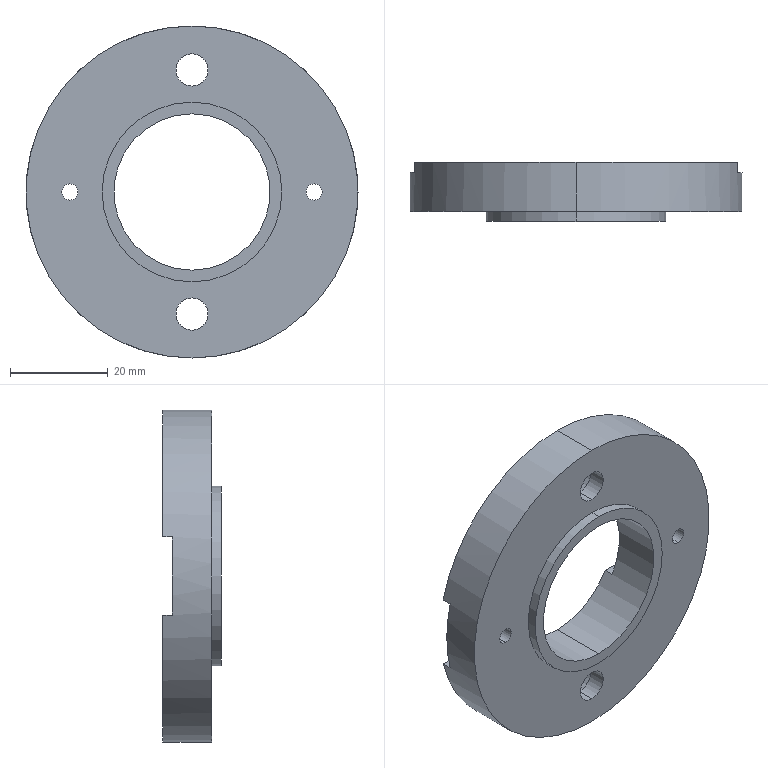Part | SolidWorks | features ICE 6, HoleWzd 2, Revolution 1 | 1 solid | 30 faces | box 68 x 12 x 68 mm | volume 26017 mm3 | cylinder 18 | plane 12 | commonest cylinder face diameters 3.3 x4 6.6 x4 11 x4 32 x2 36.8 x2 68 x2
STEP:
#1=CARTESIAN_POINT('',(-25.,36.,1.65));
#2=VERTEX_POINT('',#1);
#3=CARTESIAN_POINT('',(-25.,36.,-1.65));
#4=VERTEX_POINT('',#3);
#5=CARTESIAN_POINT('',(-25.,36.,0.));
#6=DIRECTION('',(0.,-1.,0.));
#7=DIRECTION('',(0.,0.,-1.));
#8=AXIS2_PLACEMENT_3D('',#5,#6,#7);
#9=CIRCLE('',#8,1.65);
#10=EDGE_CURVE('',#2,#4,#9,.T.);
#11=ORIENTED_EDGE('',*,*,#10,.T.);
#12=CARTESIAN_POINT('',(-25.,44.,-1.65));
#13=VERTEX_POINT('',#12);
#14=CARTESIAN_POINT('',(-25.,46.,-1.65));
#15=DIRECTION('',(0.,1.,0.));
#16=VECTOR('',#15,1000.);
#17=LINE('',#14,#16);
#18=EDGE_CURVE('',#4,#13,#17,.T.);
#19=ORIENTED_EDGE('',*,*,#18,.T.);
#20=CARTESIAN_POINT('',(-25.,44.,1.65));
#21=VERTEX_POINT('',#20);
#22=CARTESIAN_POINT('',(-25.,44.,0.));
#23=DIRECTION('',(0.,1.,0.));
#24=DIRECTION('',(0.,0.,1.));
#25=AXIS2_PLACEMENT_3D('',#22,#23,#24);
#26=CIRCLE('',#25,1.65);
#27=EDGE_CURVE('',#13,#21,#26,.T.);
#28=ORIENTED_EDGE('',*,*,#27,.T.);
#29=CARTESIAN_POINT('',(-25.,46.,1.65));
#30=DIRECTION('',(0.,1.,0.));
#31=VECTOR('',#30,1000.);
#32=LINE('',#29,#31);
#33=EDGE_CURVE('',#2,#21,#32,.T.);
#34=ORIENTED_EDGE('',*,*,#33,.F.);
#35=EDGE_LOOP('',(#11,#19,#28,#34));
#36=FACE_OUTER_BOUND('',#35,.T.);
#37=CARTESIAN_POINT('',(-25.,46.,0.));
#38=DIRECTION('',(0.,1.,0.));
#39=DIRECTION('',(0.,0.,1.));
#40=AXIS2_PLACEMENT_3D('',#37,#38,#39);
#41=CYLINDRICAL_SURFACE('',#40,1.65);
#42=ADVANCED_FACE('',(#36),#41,.F.);
#43=CARTESIAN_POINT('',(25.,36.,1.65));
#44=VERTEX_POINT('',#43);
#45=CARTESIAN_POINT('',(25.,36.,-1.65));
#46=VERTEX_POINT('',#45);
#47=CARTESIAN_POINT('',(25.,36.,0.));
#48=DIRECTION('',(0.,-1.,0.));
#49=DIRECTION('',(0.,0.,-1.));
#50=AXIS2_PLACEMENT_3D('',#47,#48,#49);
#51=CIRCLE('',#50,1.65);
#52=EDGE_CURVE('',#44,#46,#51,.T.);
#53=ORIENTED_EDGE('',*,*,#52,.T.);
#54=CARTESIAN_POINT('',(25.,44.,-1.65));
#55=VERTEX_POINT('',#54);
#56=CARTESIAN_POINT('',(25.,46.,-1.65));
#57=DIRECTION('',(0.,1.,0.));
#58=VECTOR('',#57,1000.);
#59=LINE('',#56,#58);
#60=EDGE_CURVE('',#46,#55,#59,.T.);
#61=ORIENTED_EDGE('',*,*,#60,.T.);
#62=CARTESIAN_POINT('',(25.,44.,1.65));
#63=VERTEX_POINT('',#62);
#64=CARTESIAN_POINT('',(25.,44.,0.));
#65=DIRECTION('',(0.,1.,0.));
#66=DIRECTION('',(0.,0.,1.));
#67=AXIS2_PLACEMENT_3D('',#64,#65,#66);
#68=CIRCLE('',#67,1.65);
#69=EDGE_CURVE('',#55,#63,#68,.T.);
#70=ORIENTED_EDGE('',*,*,#69,.T.);
#71=CARTESIAN_POINT('',(25.,46.,1.65));
#72=DIRECTION('',(0.,1.,0.));
#73=VECTOR('',#72,1000.);
#74=LINE('',#71,#73);
#75=EDGE_CURVE('',#44,#63,#74,.T.);
#76=ORIENTED_EDGE('',*,*,#75,.F.);
#77=EDGE_LOOP('',(#53,#61,#70,#76));
#78=FACE_OUTER_BOUND('',#77,.T.);
#79=CARTESIAN_POINT('',(25.,46.,0.));
#80=DIRECTION('',(0.,1.,0.));
#81=DIRECTION('',(0.,0.,1.));
#82=AXIS2_PLACEMENT_3D('',#79,#80,#81);
#83=CYLINDRICAL_SURFACE('',#82,1.65);
#84=ADVANCED_FACE('',(#78),#83,.F.);
#85=CARTESIAN_POINT('',(0.,39.6,-30.5));
#86=VERTEX_POINT('',#85);
#87=CARTESIAN_POINT('',(0.,39.6,-19.5));
#88=VERTEX_POINT('',#87);
#89=CARTESIAN_POINT('',(0.,39.6,-25.));
#90=DIRECTION('',(0.,1.,0.));
#91=DIRECTION('',(0.,0.,1.));
#92=AXIS2_PLACEMENT_3D('',#89,#90,#91);
#93=CIRCLE('',#92,5.5);
#94=EDGE_CURVE('',#86,#88,#93,.T.);
#95=ORIENTED_EDGE('',*,*,#94,.F.);
#96=CARTESIAN_POINT('',(0.,46.,-30.5));
#97=VERTEX_POINT('',#96);
#98=CARTESIAN_POINT('',(0.,46.,-30.5));
#99=DIRECTION('',(0.,1.,0.));
#100=VECTOR('',#99,1000.);
#101=LINE('',#98,#100);
#102=EDGE_CURVE('',#86,#97,#101,.T.);
#103=ORIENTED_EDGE('',*,*,#102,.T.);
#104=CARTESIAN_POINT('',(0.,46.,-19.5));
#105=VERTEX_POINT('',#104);
#106=CARTESIAN_POINT('',(0.,46.,-25.));
#107=DIRECTION('',(0.,1.,0.));
#108=DIRECTION('',(0.,0.,1.));
#109=AXIS2_PLACEMENT_3D('',#106,#107,#108);
#110=CIRCLE('',#109,5.5);
#111=EDGE_CURVE('',#97,#105,#110,.T.);
#112=ORIENTED_EDGE('',*,*,#111,.T.);
#113=CARTESIAN_POINT('',(0.,46.,-19.5));
#114=DIRECTION('',(0.,1.,0.));
#115=VECTOR('',#114,1000.);
#116=LINE('',#113,#115);
#117=EDGE_CURVE('',#88,#105,#116,.T.);
#118=ORIENTED_EDGE('',*,*,#117,.F.);
#119=EDGE_LOOP('',(#95,#103,#112,#118));
#120=FACE_OUTER_BOUND('',#119,.T.);
#121=CARTESIAN_POINT('',(0.,46.,-25.));
#122=DIRECTION('',(0.,1.,0.));
#123=DIRECTION('',(0.,0.,1.));
#124=AXIS2_PLACEMENT_3D('',#121,#122,#123);
#125=CYLINDRICAL_SURFACE('',#124,5.5);
#126=ADVANCED_FACE('',(#120),#125,.F.);
#127=CARTESIAN_POINT('',(0.,36.,-21.7));
#128=VERTEX_POINT('',#127);
#129=CARTESIAN_POINT('',(0.,36.,-28.3));
#130=VERTEX_POINT('',#129);
#131=CARTESIAN_POINT('',(0.,36.,-25.));
#132=DIRECTION('',(0.,-1.,0.));
#133=DIRECTION('',(0.,0.,-1.));
#134=AXIS2_PLACEMENT_3D('',#131,#132,#133);
#135=CIRCLE('',#134,3.3);
#136=EDGE_CURVE('',#128,#130,#135,.T.);
#137=ORIENTED_EDGE('',*,*,#136,.T.);
#138=CARTESIAN_POINT('',(0.,39.6,-28.3));
#139=VERTEX_POINT('',#138);
#140=CARTESIAN_POINT('',(0.,46.,-28.3));
#141=DIRECTION('',(0.,1.,0.));
#142=VECTOR('',#141,1000.);
#143=LINE('',#140,#142);
#144=EDGE_CURVE('',#130,#139,#143,.T.);
#145=ORIENTED_EDGE('',*,*,#144,.T.);
#146=CARTESIAN_POINT('',(0.,39.6,-21.7));
#147=VERTEX_POINT('',#146);
#148=CARTESIAN_POINT('',(0.,39.6,-25.));
#149=DIRECTION('',(0.,1.,0.));
#150=DIRECTION('',(0.,0.,1.));
#151=AXIS2_PLACEMENT_3D('',#148,#149,#150);
#152=CIRCLE('',#151,3.3);
#153=EDGE_CURVE('',#139,#147,#152,.T.);
#154=ORIENTED_EDGE('',*,*,#153,.T.);
#155=CARTESIAN_POINT('',(0.,46.,-21.7));
#156=DIRECTION('',(0.,1.,0.));
#157=VECTOR('',#156,1000.);
#158=LINE('',#155,#157);
#159=EDGE_CURVE('',#128,#147,#158,.T.);
#160=ORIENTED_EDGE('',*,*,#159,.F.);
#161=EDGE_LOOP('',(#137,#145,#154,#160));
#162=FACE_OUTER_BOUND('',#161,.T.);
#163=CARTESIAN_POINT('',(0.,46.,-25.));
#164=DIRECTION('',(0.,1.,0.));
#165=DIRECTION('',(0.,0.,1.));
#166=AXIS2_PLACEMENT_3D('',#163,#164,#165);
#167=CYLINDRICAL_SURFACE('',#166,3.3);
#168=ADVANCED_FACE('',(#162),#167,.F.);
#169=CARTESIAN_POINT('',(0.,39.6,19.5));
#170=VERTEX_POINT('',#169);
#171=CARTESIAN_POINT('',(0.,39.6,30.5));
#172=VERTEX_POINT('',#171);
#173=CARTESIAN_POINT('',(0.,39.6,25.));
#174=DIRECTION('',(0.,1.,0.));
#175=DIRECTION('',(0.,0.,1.));
#176=AXIS2_PLACEMENT_3D('',#173,#174,#175);
#177=CIRCLE('',#176,5.5);
#178=EDGE_CURVE('',#170,#172,#177,.T.);
#179=ORIENTED_EDGE('',*,*,#178,.F.);
#180=CARTESIAN_POINT('',(0.,46.,19.5));
#181=VERTEX_POINT('',#180);
#182=CARTESIAN_POINT('',(0.,46.,19.5));
#183=DIRECTION('',(0.,1.,0.));
#184=VECTOR('',#183,1000.);
#185=LINE('',#182,#184);
#186=EDGE_CURVE('',#170,#181,#185,.T.);
#187=ORIENTED_EDGE('',*,*,#186,.T.);
#188=CARTESIAN_POINT('',(0.,46.,30.5));
#189=VERTEX_POINT('',#188);
#190=CARTESIAN_POINT('',(0.,46.,25.));
#191=DIRECTION('',(0.,1.,0.));
#192=DIRECTION('',(0.,0.,1.));
#193=AXIS2_PLACEMENT_3D('',#190,#191,#192);
#194=CIRCLE('',#193,5.5);
#195=EDGE_CURVE('',#181,#189,#194,.T.);
#196=ORIENTED_EDGE('',*,*,#195,.T.);
#197=CARTESIAN_POINT('',(0.,46.,30.5));
#198=DIRECTION('',(0.,1.,0.));
#199=VECTOR('',#198,1000.);
#200=LINE('',#197,#199);
#201=EDGE_CURVE('',#172,#189,#200,.T.);
#202=ORIENTED_EDGE('',*,*,#201,.F.);
#203=EDGE_LOOP('',(#179,#187,#196,#202));
#204=FACE_OUTER_BOUND('',#203,.T.);
#205=CARTESIAN_POINT('',(0.,46.,25.));
#206=DIRECTION('',(0.,1.,0.));
#207=DIRECTION('',(0.,0.,1.));
#208=AXIS2_PLACEMENT_3D('',#205,#206,#207);
#209=CYLINDRICAL_SURFACE('',#208,5.5);
#210=ADVANCED_FACE('',(#204),#209,.F.);
#211=CARTESIAN_POINT('',(0.,36.,28.3));
#212=VERTEX_POINT('',#211);
#213=CARTESIAN_POINT('',(0.,36.,21.7));
#214=VERTEX_POINT('',#213);
#215=CARTESIAN_POINT('',(0.,36.,25.));
#216=DIRECTION('',(0.,-1.,0.));
#217=DIRECTION('',(0.,0.,-1.));
#218=AXIS2_PLACEMENT_3D('',#215,#216,#217);
#219=CIRCLE('',#218,3.3);
#220=EDGE_CURVE('',#212,#214,#219,.T.);
#221=ORIENTED_EDGE('',*,*,#220,.T.);
#222=CARTESIAN_POINT('',(0.,39.6,21.7));
#223=VERTEX_POINT('',#222);
#224=CARTESIAN_POINT('',(0.,46.,21.7));
#225=DIRECTION('',(0.,1.,0.));
#226=VECTOR('',#225,1000.);
#227=LINE('',#224,#226);
#228=EDGE_CURVE('',#214,#223,#227,.T.);
#229=ORIENTED_EDGE('',*,*,#228,.T.);
#230=CARTESIAN_POINT('',(0.,39.6,28.3));
#231=VERTEX_POINT('',#230);
#232=CARTESIAN_POINT('',(0.,39.6,25.));
#233=DIRECTION('',(0.,1.,0.));
#234=DIRECTION('',(0.,0.,1.));
#235=AXIS2_PLACEMENT_3D('',#232,#233,#234);
#236=CIRCLE('',#235,3.3);
#237=EDGE_CURVE('',#223,#231,#236,.T.);
#238=ORIENTED_EDGE('',*,*,#237,.T.);
#239=CARTESIAN_POINT('',(0.,46.,28.3));
#240=DIRECTION('',(0.,1.,0.));
#241=VECTOR('',#240,1000.);
#242=LINE('',#239,#241);
#243=EDGE_CURVE('',#212,#231,#242,.T.);
#244=ORIENTED_EDGE('',*,*,#243,.F.);
#245=EDGE_LOOP('',(#221,#229,#238,#244));
#246=FACE_OUTER_BOUND('',#245,.T.);
#247=CARTESIAN_POINT('',(0.,46.,25.));
#248=DIRECTION('',(0.,1.,0.));
#249=DIRECTION('',(0.,0.,1.));
#250=AXIS2_PLACEMENT_3D('',#247,#248,#249);
#251=CYLINDRICAL_SURFACE('',#250,3.3);
#252=ADVANCED_FACE('',(#246),#251,.F.);
#253=CARTESIAN_POINT('',(33.045,46.,8.));
#254=VERTEX_POINT('',#253);
#255=CARTESIAN_POINT('',(0.,46.,34.));
#256=VERTEX_POINT('',#255);
#257=CARTESIAN_POINT('',(0.,46.,0.));
#258=DIRECTION('',(0.,-1.,0.));
#259=DIRECTION('',(0.,0.,-1.));
#260=AXIS2_PLACEMENT_3D('',#257,#258,#259);
#261=CIRCLE('',#260,34.);
#262=EDGE_CURVE('',#254,#256,#261,.T.);
#263=ORIENTED_EDGE('',*,*,#262,.T.);
#264=CARTESIAN_POINT('',(0.,36.,34.));
#265=VERTEX_POINT('',#264);
#266=CARTESIAN_POINT('',(0.,0.,34.));
#267=DIRECTION('',(0.,-1.,0.));
#268=VECTOR('',#267,1000.);
#269=LINE('',#266,#268);
#270=EDGE_CURVE('',#256,#265,#269,.T.);
#271=ORIENTED_EDGE('',*,*,#270,.T.);
#272=CARTESIAN_POINT('',(0.,36.,-34.));
#273=VERTEX_POINT('',#272);
#274=CARTESIAN_POINT('',(0.,36.,0.));
#275=DIRECTION('',(0.,-1.,0.));
#276=DIRECTION('',(0.,0.,-1.));
#277=AXIS2_PLACEMENT_3D('',#274,#275,#276);
#278=CIRCLE('',#277,34.);
#279=EDGE_CURVE('',#273,#265,#278,.T.);
#280=ORIENTED_EDGE('',*,*,#279,.F.);
#281=CARTESIAN_POINT('',(0.,46.,-34.));
#282=VERTEX_POINT('',#281);
#283=CARTESIAN_POINT('',(0.,0.,-34.));
#284=DIRECTION('',(0.,-1.,0.));
#285=VECTOR('',#284,1000.);
#286=LINE('',#283,#285);
#287=EDGE_CURVE('',#282,#273,#286,.T.);
#288=ORIENTED_EDGE('',*,*,#287,.F.);
#289=CARTESIAN_POINT('',(33.045,46.,-8.));
#290=VERTEX_POINT('',#289);
#291=CARTESIAN_POINT('',(0.,46.,0.));
#292=DIRECTION('',(0.,-1.,0.));
#293=DIRECTION('',(0.,0.,-1.));
#294=AXIS2_PLACEMENT_3D('',#291,#292,#293);
#295=CIRCLE('',#294,34.);
#296=EDGE_CURVE('',#282,#290,#295,.T.);
#297=ORIENTED_EDGE('',*,*,#296,.T.);
#298=CARTESIAN_POINT('',(33.045,44.,-8.));
#299=VERTEX_POINT('',#298);
#300=CARTESIAN_POINT('',(33.045,0.,-8.));
#301=DIRECTION('',(0.,1.,0.));
#302=VECTOR('',#301,1000.);
#303=LINE('',#300,#302);
#304=EDGE_CURVE('',#299,#290,#303,.T.);
#305=ORIENTED_EDGE('',*,*,#304,.F.);
#306=CARTESIAN_POINT('',(33.045,44.,8.));
#307=VERTEX_POINT('',#306);
#308=CARTESIAN_POINT('',(0.,44.,0.));
#309=DIRECTION('',(0.,-1.,0.));
#310=DIRECTION('',(0.,0.,1.));
#311=AXIS2_PLACEMENT_3D('',#308,#309,#310);
#312=CIRCLE('',#311,34.);
#313=EDGE_CURVE('',#299,#307,#312,.T.);
#314=ORIENTED_EDGE('',*,*,#313,.T.);
#315=CARTESIAN_POINT('',(33.045,0.,8.));
#316=DIRECTION('',(0.,-1.,0.));
#317=VECTOR('',#316,1000.);
#318=LINE('',#315,#317);
#319=EDGE_CURVE('',#254,#307,#318,.T.);
#320=ORIENTED_EDGE('',*,*,#319,.F.);
#321=EDGE_LOOP('',(#263,#271,#280,#288,#297,#305,#314,#320));
#322=FACE_OUTER_BOUND('',#321,.T.);
#323=CARTESIAN_POINT('',(0.,0.,0.));
#324=DIRECTION('',(0.,-1.,0.));
#325=DIRECTION('',(0.,0.,-1.));
#326=AXIS2_PLACEMENT_3D('',#323,#324,#325);
#327=CYLINDRICAL_SURFACE('',#326,34.);
#328=ADVANCED_FACE('',(#322),#327,.T.);
#329=CARTESIAN_POINT('',(0.,36.,-18.4));
#330=VERTEX_POINT('',#329);
#331=CARTESIAN_POINT('',(0.,36.,18.4));
#332=VERTEX_POINT('',#331);
#333=CARTESIAN_POINT('',(0.,36.,0.));
#334=DIRECTION('',(0.,-1.,0.));
#335=DIRECTION('',(0.,0.,-1.));
#336=AXIS2_PLACEMENT_3D('',#333,#334,#335);
#337=CIRCLE('',#336,18.4);
#338=EDGE_CURVE('',#330,#332,#337,.T.);
#339=ORIENTED_EDGE('',*,*,#338,.T.);
#340=CARTESIAN_POINT('',(0.,34.,18.4));
#341=VERTEX_POINT('',#340);
#342=CARTESIAN_POINT('',(0.,0.,18.4));
#343=DIRECTION('',(0.,-1.,0.));
#344=VECTOR('',#343,1000.);
#345=LINE('',#342,#344);
#346=EDGE_CURVE('',#332,#341,#345,.T.);
#347=ORIENTED_EDGE('',*,*,#346,.T.);
#348=CARTESIAN_POINT('',(0.,34.,-18.4));
#349=VERTEX_POINT('',#348);
#350=CARTESIAN_POINT('',(0.,34.,0.));
#351=DIRECTION('',(0.,1.,0.));
#352=DIRECTION('',(0.,0.,-1.));
#353=AXIS2_PLACEMENT_3D('',#350,#351,#352);
#354=CIRCLE('',#353,18.4);
#355=EDGE_CURVE('',#341,#349,#354,.T.);
#356=ORIENTED_EDGE('',*,*,#355,.T.);
#357=CARTESIAN_POINT('',(0.,0.,-18.4));
#358=DIRECTION('',(0.,-1.,0.));
#359=VECTOR('',#358,1000.);
#360=LINE('',#357,#359);
#361=EDGE_CURVE('',#330,#349,#360,.T.);
#362=ORIENTED_EDGE('',*,*,#361,.F.);
#363=EDGE_LOOP('',(#339,#347,#356,#362));
#364=FACE_OUTER_BOUND('',#363,.T.);
#365=CARTESIAN_POINT('',(0.,0.,0.));
#366=DIRECTION('',(0.,-1.,0.));
#367=DIRECTION('',(0.,0.,-1.));
#368=AXIS2_PLACEMENT_3D('',#365,#366,#367);
#369=CYLINDRICAL_SURFACE('',#368,18.4);
#370=ADVANCED_FACE('',(#364),#369,.T.);
#371=CARTESIAN_POINT('',(0.,34.,-16.));
#372=VERTEX_POINT('',#371);
#373=CARTESIAN_POINT('',(0.,34.,16.));
#374=VERTEX_POINT('',#373);
#375=CARTESIAN_POINT('',(0.,34.,0.));
#376=DIRECTION('',(0.,1.,0.));
#377=DIRECTION('',(0.,0.,-1.));
#378=AXIS2_PLACEMENT_3D('',#375,#376,#377);
#379=CIRCLE('',#378,16.);
#380=EDGE_CURVE('',#372,#374,#379,.T.);
#381=ORIENTED_EDGE('',*,*,#380,.F.);
#382=CARTESIAN_POINT('',(0.,46.,-16.));
#383=VERTEX_POINT('',#382);
#384=CARTESIAN_POINT('',(0.,0.,-16.));
#385=DIRECTION('',(0.,1.,0.));
#386=VECTOR('',#385,1000.);
#387=LINE('',#384,#386);
#388=EDGE_CURVE('',#372,#383,#387,.T.);
#389=ORIENTED_EDGE('',*,*,#388,.T.);
#390=CARTESIAN_POINT('',(-13.856,46.,-8.));
#391=VERTEX_POINT('',#390);
#392=CARTESIAN_POINT('',(0.,46.,0.));
#393=DIRECTION('',(0.,1.,0.));
#394=DIRECTION('',(0.,0.,1.));
#395=AXIS2_PLACEMENT_3D('',#392,#393,#394);
#396=CIRCLE('',#395,16.);
#397=EDGE_CURVE('',#383,#391,#396,.T.);
#398=ORIENTED_EDGE('',*,*,#397,.T.);
#399=CARTESIAN_POINT('',(-13.856,44.,-8.));
#400=VERTEX_POINT('',#399);
#401=CARTESIAN_POINT('',(-13.856,0.,-8.));
#402=DIRECTION('',(0.,-1.,0.));
#403=VECTOR('',#402,1000.);
#404=LINE('',#401,#403);
#405=EDGE_CURVE('',#391,#400,#404,.T.);
#406=ORIENTED_EDGE('',*,*,#405,.T.);
#407=CARTESIAN_POINT('',(-13.856,44.,8.));
#408=VERTEX_POINT('',#407);
#409=CARTESIAN_POINT('',(0.,44.,0.));
#410=DIRECTION('',(0.,-1.,0.));
#411=DIRECTION('',(0.,0.,1.));
#412=AXIS2_PLACEMENT_3D('',#409,#410,#411);
#413=CIRCLE('',#412,16.);
#414=EDGE_CURVE('',#408,#400,#413,.T.);
#415=ORIENTED_EDGE('',*,*,#414,.F.);
#416=CARTESIAN_POINT('',(-13.856,46.,8.));
#417=VERTEX_POINT('',#416);
#418=CARTESIAN_POINT('',(-13.856,0.,8.));
#419=DIRECTION('',(0.,1.,0.));
#420=VECTOR('',#419,1000.);
#421=LINE('',#418,#420);
#422=EDGE_CURVE('',#408,#417,#421,.T.);
#423=ORIENTED_EDGE('',*,*,#422,.T.);
#424=CARTESIAN_POINT('',(0.,46.,16.));
#425=VERTEX_POINT('',#424);
#426=CARTESIAN_POINT('',(0.,46.,0.));
#427=DIRECTION('',(0.,1.,0.));
#428=DIRECTION('',(0.,0.,1.));
#429=AXIS2_PLACEMENT_3D('',#426,#427,#428);
#430=CIRCLE('',#429,16.);
#431=EDGE_CURVE('',#417,#425,#430,.T.);
#432=ORIENTED_EDGE('',*,*,#431,.T.);
#433=CARTESIAN_POINT('',(0.,0.,16.));
#434=DIRECTION('',(0.,1.,0.));
#435=VECTOR('',#434,1000.);
#436=LINE('',#433,#435);
#437=EDGE_CURVE('',#374,#425,#436,.T.);
#438=ORIENTED_EDGE('',*,*,#437,.F.);
#439=EDGE_LOOP('',(#381,#389,#398,#406,#415,#423,#432,#438));
#440=FACE_OUTER_BOUND('',#439,.T.);
#441=CARTESIAN_POINT('',(0.,0.,0.));
#442=DIRECTION('',(0.,1.,0.));
#443=DIRECTION('',(0.,0.,1.));
#444=AXIS2_PLACEMENT_3D('',#441,#442,#443);
#445=CYLINDRICAL_SURFACE('',#444,16.);
#446=ADVANCED_FACE('',(#440),#445,.F.);
#447=ORIENTED_EDGE('',*,*,#431,.F.);
#448=CARTESIAN_POINT('',(-33.045,46.,8.));
#449=VERTEX_POINT('',#448);
#450=CARTESIAN_POINT('',(-33.045,46.,8.));
#451=DIRECTION('',(1.,0.,0.));
#452=VECTOR('',#451,1000.);
#453=LINE('',#450,#452);
#454=EDGE_CURVE('',#449,#417,#453,.T.);
#455=ORIENTED_EDGE('',*,*,#454,.F.);
#456=CARTESIAN_POINT('',(0.,46.,0.));
#457=DIRECTION('',(0.,-1.,0.));
#458=DIRECTION('',(0.,0.,-1.));
#459=AXIS2_PLACEMENT_3D('',#456,#457,#458);
#460=CIRCLE('',#459,34.);
#461=EDGE_CURVE('',#256,#449,#460,.T.);
#462=ORIENTED_EDGE('',*,*,#461,.F.);
#463=ORIENTED_EDGE('',*,*,#262,.F.);
#464=CARTESIAN_POINT('',(13.856,46.,8.));
#465=VERTEX_POINT('',#464);
#466=CARTESIAN_POINT('',(33.045,46.,8.));
#467=DIRECTION('',(1.,0.,0.));
#468=VECTOR('',#467,1000.);
#469=LINE('',#466,#468);
#470=EDGE_CURVE('',#465,#254,#469,.T.);
#471=ORIENTED_EDGE('',*,*,#470,.F.);
#472=CARTESIAN_POINT('',(0.,46.,0.));
#473=DIRECTION('',(0.,1.,0.));
#474=DIRECTION('',(0.,0.,1.));
#475=AXIS2_PLACEMENT_3D('',#472,#473,#474);
#476=CIRCLE('',#475,16.);
#477=EDGE_CURVE('',#425,#465,#476,.T.);
#478=ORIENTED_EDGE('',*,*,#477,.F.);
#479=EDGE_LOOP('',(#447,#455,#462,#463,#471,#478));
#480=FACE_OUTER_BOUND('',#479,.T.);
#481=CARTESIAN_POINT('',(0.,46.,25.));
#482=DIRECTION('',(0.,1.,0.));
#483=DIRECTION('',(0.,0.,1.));
#484=AXIS2_PLACEMENT_3D('',#481,#482,#483);
#485=CIRCLE('',#484,5.5);
#486=EDGE_CURVE('',#189,#181,#485,.T.);
#487=ORIENTED_EDGE('',*,*,#486,.F.);
#488=ORIENTED_EDGE('',*,*,#195,.F.);
#489=EDGE_LOOP('',(#487,#488));
#490=FACE_BOUND('',#489,.T.);
#491=CARTESIAN_POINT('',(0.,46.,0.));
#492=DIRECTION('',(0.,1.,0.));
#493=DIRECTION('',(0.,0.,1.));
#494=AXIS2_PLACEMENT_3D('',#491,#492,#493);
#495=PLANE('',#494);
#496=ADVANCED_FACE('',(#480,#490),#495,.T.);
#497=ORIENTED_EDGE('',*,*,#388,.F.);
#498=CARTESIAN_POINT('',(0.,34.,0.));
#499=DIRECTION('',(0.,1.,0.));
#500=DIRECTION('',(0.,0.,-1.));
#501=AXIS2_PLACEMENT_3D('',#498,#499,#500);
#502=CIRCLE('',#501,16.);
#503=EDGE_CURVE('',#374,#372,#502,.T.);
#504=ORIENTED_EDGE('',*,*,#503,.F.);
#505=ORIENTED_EDGE('',*,*,#437,.T.);
#506=ORIENTED_EDGE('',*,*,#477,.T.);
#507=CARTESIAN_POINT('',(13.856,44.,8.));
#508=VERTEX_POINT('',#507);
#509=CARTESIAN_POINT('',(13.856,0.,8.));
#510=DIRECTION('',(0.,-1.,0.));
#511=VECTOR('',#510,1000.);
#512=LINE('',#509,#511);
#513=EDGE_CURVE('',#465,#508,#512,.T.);
#514=ORIENTED_EDGE('',*,*,#513,.T.);
#515=CARTESIAN_POINT('',(13.856,44.,-8.));
#516=VERTEX_POINT('',#515);
#517=CARTESIAN_POINT('',(0.,44.,0.));
#518=DIRECTION('',(0.,-1.,0.));
#519=DIRECTION('',(0.,0.,1.));
#520=AXIS2_PLACEMENT_3D('',#517,#518,#519);
#521=CIRCLE('',#520,16.);
#522=EDGE_CURVE('',#516,#508,#521,.T.);
#523=ORIENTED_EDGE('',*,*,#522,.F.);
#524=CARTESIAN_POINT('',(13.856,46.,-8.));
#525=VERTEX_POINT('',#524);
#526=CARTESIAN_POINT('',(13.856,0.,-8.));
#527=DIRECTION('',(0.,1.,0.));
#528=VECTOR('',#527,1000.);
#529=LINE('',#526,#528);
#530=EDGE_CURVE('',#516,#525,#529,.T.);
#531=ORIENTED_EDGE('',*,*,#530,.T.);
#532=CARTESIAN_POINT('',(0.,46.,0.));
#533=DIRECTION('',(0.,1.,0.));
#534=DIRECTION('',(0.,0.,1.));
#535=AXIS2_PLACEMENT_3D('',#532,#533,#534);
#536=CIRCLE('',#535,16.);
#537=EDGE_CURVE('',#525,#383,#536,.T.);
#538=ORIENTED_EDGE('',*,*,#537,.T.);
#539=EDGE_LOOP('',(#497,#504,#505,#506,#514,#523,#531,#538));
#540=FACE_OUTER_BOUND('',#539,.T.);
#541=CARTESIAN_POINT('',(0.,0.,0.));
#542=DIRECTION('',(0.,1.,0.));
#543=DIRECTION('',(0.,0.,1.));
#544=AXIS2_PLACEMENT_3D('',#541,#542,#543);
#545=CYLINDRICAL_SURFACE('',#544,16.);
#546=ADVANCED_FACE('',(#540),#545,.F.);
#547=ORIENTED_EDGE('',*,*,#346,.F.);
#548=CARTESIAN_POINT('',(0.,36.,0.));
#549=DIRECTION('',(0.,-1.,0.));
#550=DIRECTION('',(0.,0.,-1.));
#551=AXIS2_PLACEMENT_3D('',#548,#549,#550);
#552=CIRCLE('',#551,18.4);
#553=EDGE_CURVE('',#332,#330,#552,.T.);
#554=ORIENTED_EDGE('',*,*,#553,.T.);
#555=ORIENTED_EDGE('',*,*,#361,.T.);
#556=CARTESIAN_POINT('',(0.,34.,0.));
#557=DIRECTION('',(0.,1.,0.));
#558=DIRECTION('',(0.,0.,-1.));
#559=AXIS2_PLACEMENT_3D('',#556,#557,#558);
#560=CIRCLE('',#559,18.4);
#561=EDGE_CURVE('',#349,#341,#560,.T.);
#562=ORIENTED_EDGE('',*,*,#561,.T.);
#563=EDGE_LOOP('',(#547,#554,#555,#562));
#564=FACE_OUTER_BOUND('',#563,.T.);
#565=CARTESIAN_POINT('',(0.,0.,0.));
#566=DIRECTION('',(0.,-1.,0.));
#567=DIRECTION('',(0.,0.,-1.));
#568=AXIS2_PLACEMENT_3D('',#565,#566,#567);
#569=CYLINDRICAL_SURFACE('',#568,18.4);
#570=ADVANCED_FACE('',(#564),#569,.T.);
#571=ORIENTED_EDGE('',*,*,#537,.F.);
#572=CARTESIAN_POINT('',(33.045,46.,-8.));
#573=DIRECTION('',(-1.,0.,0.));
#574=VECTOR('',#573,1000.);
#575=LINE('',#572,#574);
#576=EDGE_CURVE('',#290,#525,#575,.T.);
#577=ORIENTED_EDGE('',*,*,#576,.F.);
#578=ORIENTED_EDGE('',*,*,#296,.F.);
#579=CARTESIAN_POINT('',(-33.045,46.,-8.));
#580=VERTEX_POINT('',#579);
#581=CARTESIAN_POINT('',(0.,46.,0.));
#582=DIRECTION('',(0.,-1.,0.));
#583=DIRECTION('',(0.,0.,-1.));
#584=AXIS2_PLACEMENT_3D('',#581,#582,#583);
#585=CIRCLE('',#584,34.);
#586=EDGE_CURVE('',#580,#282,#585,.T.);
#587=ORIENTED_EDGE('',*,*,#586,.F.);
#588=CARTESIAN_POINT('',(-33.045,46.,-8.));
#589=DIRECTION('',(-1.,0.,0.));
#590=VECTOR('',#589,1000.);
#591=LINE('',#588,#590);
#592=EDGE_CURVE('',#391,#580,#591,.T.);
#593=ORIENTED_EDGE('',*,*,#592,.F.);
#594=ORIENTED_EDGE('',*,*,#397,.F.);
#595=EDGE_LOOP('',(#571,#577,#578,#587,#593,#594));
#596=FACE_OUTER_BOUND('',#595,.T.);
#597=CARTESIAN_POINT('',(0.,46.,-25.));
#598=DIRECTION('',(0.,1.,0.));
#599=DIRECTION('',(0.,0.,1.));
#600=AXIS2_PLACEMENT_3D('',#597,#598,#599);
#601=CIRCLE('',#600,5.5);
#602=EDGE_CURVE('',#105,#97,#601,.T.);
#603=ORIENTED_EDGE('',*,*,#602,.F.);
#604=ORIENTED_EDGE('',*,*,#111,.F.);
#605=EDGE_LOOP('',(#603,#604));
#606=FACE_BOUND('',#605,.T.);
#607=CARTESIAN_POINT('',(0.,46.,0.));
#608=DIRECTION('',(0.,1.,0.));
#609=DIRECTION('',(0.,0.,1.));
#610=AXIS2_PLACEMENT_3D('',#607,#608,#609);
#611=PLANE('',#610);
#612=ADVANCED_FACE('',(#596,#606),#611,.T.);
#613=ORIENTED_EDGE('',*,*,#270,.F.);
#614=ORIENTED_EDGE('',*,*,#461,.T.);
#615=CARTESIAN_POINT('',(-33.045,44.,8.));
#616=VERTEX_POINT('',#615);
#617=CARTESIAN_POINT('',(-33.045,0.,8.));
#618=DIRECTION('',(0.,1.,0.));
#619=VECTOR('',#618,1000.);
#620=LINE('',#617,#619);
#621=EDGE_CURVE('',#616,#449,#620,.T.);
#622=ORIENTED_EDGE('',*,*,#621,.F.);
#623=CARTESIAN_POINT('',(-33.045,44.,-8.));
#624=VERTEX_POINT('',#623);
#625=CARTESIAN_POINT('',(0.,44.,0.));
#626=DIRECTION('',(0.,-1.,0.));
#627=DIRECTION('',(0.,0.,1.));
#628=AXIS2_PLACEMENT_3D('',#625,#626,#627);
#629=CIRCLE('',#628,34.);
#630=EDGE_CURVE('',#616,#624,#629,.T.);
#631=ORIENTED_EDGE('',*,*,#630,.T.);
#632=CARTESIAN_POINT('',(-33.045,0.,-8.));
#633=DIRECTION('',(0.,-1.,0.));
#634=VECTOR('',#633,1000.);
#635=LINE('',#632,#634);
#636=EDGE_CURVE('',#580,#624,#635,.T.);
#637=ORIENTED_EDGE('',*,*,#636,.F.);
#638=ORIENTED_EDGE('',*,*,#586,.T.);
#639=ORIENTED_EDGE('',*,*,#287,.T.);
#640=CARTESIAN_POINT('',(0.,36.,0.));
#641=DIRECTION('',(0.,-1.,0.));
#642=DIRECTION('',(0.,0.,-1.));
#643=AXIS2_PLACEMENT_3D('',#640,#641,#642);
#644=CIRCLE('',#643,34.);
#645=EDGE_CURVE('',#265,#273,#644,.T.);
#646=ORIENTED_EDGE('',*,*,#645,.F.);
#647=EDGE_LOOP('',(#613,#614,#622,#631,#637,#638,#639,#646));
#648=FACE_OUTER_BOUND('',#647,.T.);
#649=CARTESIAN_POINT('',(0.,0.,0.));
#650=DIRECTION('',(0.,-1.,0.));
#651=DIRECTION('',(0.,0.,-1.));
#652=AXIS2_PLACEMENT_3D('',#649,#650,#651);
#653=CYLINDRICAL_SURFACE('',#652,34.);
#654=ADVANCED_FACE('',(#648),#653,.T.);
#655=ORIENTED_EDGE('',*,*,#10,.F.);
#656=CARTESIAN_POINT('',(-25.,36.,0.));
#657=DIRECTION('',(0.,-1.,0.));
#658=DIRECTION('',(0.,0.,-1.));
#659=AXIS2_PLACEMENT_3D('',#656,#657,#658);
#660=CIRCLE('',#659,1.65);
#661=EDGE_CURVE('',#4,#2,#660,.T.);
#662=ORIENTED_EDGE('',*,*,#661,.F.);
#663=EDGE_LOOP('',(#655,#662));
#664=FACE_BOUND('',#663,.T.);
#665=ORIENTED_EDGE('',*,*,#52,.F.);
#666=CARTESIAN_POINT('',(25.,36.,0.));
#667=DIRECTION('',(0.,-1.,0.));
#668=DIRECTION('',(0.,0.,-1.));
#669=AXIS2_PLACEMENT_3D('',#666,#667,#668);
#670=CIRCLE('',#669,1.65);
#671=EDGE_CURVE('',#46,#44,#670,.T.);
#672=ORIENTED_EDGE('',*,*,#671,.F.);
#673=EDGE_LOOP('',(#665,#672));
#674=FACE_BOUND('',#673,.T.);
#675=ORIENTED_EDGE('',*,*,#136,.F.);
#676=CARTESIAN_POINT('',(0.,36.,-25.));
#677=DIRECTION('',(0.,-1.,0.));
#678=DIRECTION('',(0.,0.,-1.));
#679=AXIS2_PLACEMENT_3D('',#676,#677,#678);
#680=CIRCLE('',#679,3.3);
#681=EDGE_CURVE('',#130,#128,#680,.T.);
#682=ORIENTED_EDGE('',*,*,#681,.F.);
#683=EDGE_LOOP('',(#675,#682));
#684=FACE_BOUND('',#683,.T.);
#685=ORIENTED_EDGE('',*,*,#220,.F.);
#686=CARTESIAN_POINT('',(0.,36.,25.));
#687=DIRECTION('',(0.,-1.,0.));
#688=DIRECTION('',(0.,0.,-1.));
#689=AXIS2_PLACEMENT_3D('',#686,#687,#688);
#690=CIRCLE('',#689,3.3);
#691=EDGE_CURVE('',#214,#212,#690,.T.);
#692=ORIENTED_EDGE('',*,*,#691,.F.);
#693=EDGE_LOOP('',(#685,#692));
#694=FACE_BOUND('',#693,.T.);
#695=ORIENTED_EDGE('',*,*,#279,.T.);
#696=ORIENTED_EDGE('',*,*,#645,.T.);
#697=EDGE_LOOP('',(#695,#696));
#698=FACE_OUTER_BOUND('',#697,.T.);
#699=ORIENTED_EDGE('',*,*,#338,.F.);
#700=ORIENTED_EDGE('',*,*,#553,.F.);
#701=EDGE_LOOP('',(#699,#700));
#702=FACE_BOUND('',#701,.T.);
#703=CARTESIAN_POINT('',(34.,36.,0.));
#704=DIRECTION('',(0.,-1.,0.));
#705=DIRECTION('',(0.,0.,-1.));
#706=AXIS2_PLACEMENT_3D('',#703,#704,#705);
#707=PLANE('',#706);
#708=ADVANCED_FACE('',(#664,#674,#684,#694,#698,#702),#707,.T.);
#709=ORIENTED_EDGE('',*,*,#228,.F.);
#710=ORIENTED_EDGE('',*,*,#691,.T.);
#711=ORIENTED_EDGE('',*,*,#243,.T.);
#712=CARTESIAN_POINT('',(0.,39.6,25.));
#713=DIRECTION('',(0.,1.,0.));
#714=DIRECTION('',(0.,0.,1.));
#715=AXIS2_PLACEMENT_3D('',#712,#713,#714);
#716=CIRCLE('',#715,3.3);
#717=EDGE_CURVE('',#231,#223,#716,.T.);
#718=ORIENTED_EDGE('',*,*,#717,.T.);
#719=EDGE_LOOP('',(#709,#710,#711,#718));
#720=FACE_OUTER_BOUND('',#719,.T.);
#721=CARTESIAN_POINT('',(0.,46.,25.));
#722=DIRECTION('',(0.,1.,0.));
#723=DIRECTION('',(0.,0.,1.));
#724=AXIS2_PLACEMENT_3D('',#721,#722,#723);
#725=CYLINDRICAL_SURFACE('',#724,3.3);
#726=ADVANCED_FACE('',(#720),#725,.F.);
#727=ORIENTED_EDGE('',*,*,#717,.F.);
#728=ORIENTED_EDGE('',*,*,#237,.F.);
#729=EDGE_LOOP('',(#727,#728));
#730=FACE_BOUND('',#729,.T.);
#731=CARTESIAN_POINT('',(0.,39.6,25.));
#732=DIRECTION('',(0.,1.,0.));
#733=DIRECTION('',(0.,0.,1.));
#734=AXIS2_PLACEMENT_3D('',#731,#732,#733);
#735=CIRCLE('',#734,5.5);
#736=EDGE_CURVE('',#172,#170,#735,.T.);
#737=ORIENTED_EDGE('',*,*,#736,.T.);
#738=ORIENTED_EDGE('',*,*,#178,.T.);
#739=EDGE_LOOP('',(#737,#738));
#740=FACE_OUTER_BOUND('',#739,.T.);
#741=CARTESIAN_POINT('',(3.3,39.6,25.));
#742=DIRECTION('',(0.,-1.,0.));
#743=DIRECTION('',(0.,0.,-1.));
#744=AXIS2_PLACEMENT_3D('',#741,#742,#743);
#745=PLANE('',#744);
#746=ADVANCED_FACE('',(#730,#740),#745,.F.);
#747=ORIENTED_EDGE('',*,*,#186,.F.);
#748=ORIENTED_EDGE('',*,*,#736,.F.);
#749=ORIENTED_EDGE('',*,*,#201,.T.);
#750=ORIENTED_EDGE('',*,*,#486,.T.);
#751=EDGE_LOOP('',(#747,#748,#749,#750));
#752=FACE_OUTER_BOUND('',#751,.T.);
#753=CARTESIAN_POINT('',(0.,46.,25.));
#754=DIRECTION('',(0.,1.,0.));
#755=DIRECTION('',(0.,0.,1.));
#756=AXIS2_PLACEMENT_3D('',#753,#754,#755);
#757=CYLINDRICAL_SURFACE('',#756,5.5);
#758=ADVANCED_FACE('',(#752),#757,.F.);
#759=ORIENTED_EDGE('',*,*,#144,.F.);
#760=ORIENTED_EDGE('',*,*,#681,.T.);
#761=ORIENTED_EDGE('',*,*,#159,.T.);
#762=CARTESIAN_POINT('',(0.,39.6,-25.));
#763=DIRECTION('',(0.,1.,0.));
#764=DIRECTION('',(0.,0.,1.));
#765=AXIS2_PLACEMENT_3D('',#762,#763,#764);
#766=CIRCLE('',#765,3.3);
#767=EDGE_CURVE('',#147,#139,#766,.T.);
#768=ORIENTED_EDGE('',*,*,#767,.T.);
#769=EDGE_LOOP('',(#759,#760,#761,#768));
#770=FACE_OUTER_BOUND('',#769,.T.);
#771=CARTESIAN_POINT('',(0.,46.,-25.));
#772=DIRECTION('',(0.,1.,0.));
#773=DIRECTION('',(0.,0.,1.));
#774=AXIS2_PLACEMENT_3D('',#771,#772,#773);
#775=CYLINDRICAL_SURFACE('',#774,3.3);
#776=ADVANCED_FACE('',(#770),#775,.F.);
#777=ORIENTED_EDGE('',*,*,#767,.F.);
#778=ORIENTED_EDGE('',*,*,#153,.F.);
#779=EDGE_LOOP('',(#777,#778));
#780=FACE_BOUND('',#779,.T.);
#781=CARTESIAN_POINT('',(0.,39.6,-25.));
#782=DIRECTION('',(0.,1.,0.));
#783=DIRECTION('',(0.,0.,1.));
#784=AXIS2_PLACEMENT_3D('',#781,#782,#783);
#785=CIRCLE('',#784,5.5);
#786=EDGE_CURVE('',#88,#86,#785,.T.);
#787=ORIENTED_EDGE('',*,*,#786,.T.);
#788=ORIENTED_EDGE('',*,*,#94,.T.);
#789=EDGE_LOOP('',(#787,#788));
#790=FACE_OUTER_BOUND('',#789,.T.);
#791=CARTESIAN_POINT('',(3.3,39.6,-25.));
#792=DIRECTION('',(0.,-1.,0.));
#793=DIRECTION('',(0.,0.,-1.));
#794=AXIS2_PLACEMENT_3D('',#791,#792,#793);
#795=PLANE('',#794);
#796=ADVANCED_FACE('',(#780,#790),#795,.F.);
#797=ORIENTED_EDGE('',*,*,#102,.F.);
#798=ORIENTED_EDGE('',*,*,#786,.F.);
#799=ORIENTED_EDGE('',*,*,#117,.T.);
#800=ORIENTED_EDGE('',*,*,#602,.T.);
#801=EDGE_LOOP('',(#797,#798,#799,#800));
#802=FACE_OUTER_BOUND('',#801,.T.);
#803=CARTESIAN_POINT('',(0.,46.,-25.));
#804=DIRECTION('',(0.,1.,0.));
#805=DIRECTION('',(0.,0.,1.));
#806=AXIS2_PLACEMENT_3D('',#803,#804,#805);
#807=CYLINDRICAL_SURFACE('',#806,5.5);
#808=ADVANCED_FACE('',(#802),#807,.F.);
#809=ORIENTED_EDGE('',*,*,#561,.F.);
#810=ORIENTED_EDGE('',*,*,#355,.F.);
#811=EDGE_LOOP('',(#809,#810));
#812=FACE_OUTER_BOUND('',#811,.T.);
#813=ORIENTED_EDGE('',*,*,#503,.T.);
#814=ORIENTED_EDGE('',*,*,#380,.T.);
#815=EDGE_LOOP('',(#813,#814));
#816=FACE_BOUND('',#815,.T.);
#817=CARTESIAN_POINT('',(34.,34.,0.));
#818=DIRECTION('',(0.,-1.,0.));
#819=DIRECTION('',(0.,0.,-1.));
#820=AXIS2_PLACEMENT_3D('',#817,#818,#819);
#821=PLANE('',#820);
#822=ADVANCED_FACE('',(#812,#816),#821,.T.);
#823=CARTESIAN_POINT('',(25.,44.,0.));
#824=DIRECTION('',(0.,1.,0.));
#825=DIRECTION('',(0.,0.,1.));
#826=AXIS2_PLACEMENT_3D('',#823,#824,#825);
#827=CIRCLE('',#826,1.65);
#828=EDGE_CURVE('',#63,#55,#827,.T.);
#829=ORIENTED_EDGE('',*,*,#828,.F.);
#830=ORIENTED_EDGE('',*,*,#69,.F.);
#831=EDGE_LOOP('',(#829,#830));
#832=FACE_BOUND('',#831,.T.);
#833=ORIENTED_EDGE('',*,*,#522,.T.);
#834=CARTESIAN_POINT('',(-50.,44.,8.));
#835=DIRECTION('',(-1.,0.,0.));
#836=VECTOR('',#835,1000.);
#837=LINE('',#834,#836);
#838=EDGE_CURVE('',#307,#508,#837,.T.);
#839=ORIENTED_EDGE('',*,*,#838,.F.);
#840=ORIENTED_EDGE('',*,*,#313,.F.);
#841=CARTESIAN_POINT('',(-50.,44.,-8.));
#842=DIRECTION('',(1.,0.,0.));
#843=VECTOR('',#842,1000.);
#844=LINE('',#841,#843);
#845=EDGE_CURVE('',#516,#299,#844,.T.);
#846=ORIENTED_EDGE('',*,*,#845,.F.);
#847=EDGE_LOOP('',(#833,#839,#840,#846));
#848=FACE_OUTER_BOUND('',#847,.T.);
#849=CARTESIAN_POINT('',(0.,44.,0.));
#850=DIRECTION('',(0.,1.,0.));
#851=DIRECTION('',(0.,0.,1.));
#852=AXIS2_PLACEMENT_3D('',#849,#850,#851);
#853=PLANE('',#852);
#854=ADVANCED_FACE('',(#832,#848),#853,.T.);
#855=ORIENTED_EDGE('',*,*,#576,.T.);
#856=ORIENTED_EDGE('',*,*,#530,.F.);
#857=ORIENTED_EDGE('',*,*,#845,.T.);
#858=ORIENTED_EDGE('',*,*,#304,.T.);
#859=EDGE_LOOP('',(#855,#856,#857,#858));
#860=FACE_OUTER_BOUND('',#859,.T.);
#861=CARTESIAN_POINT('',(-50.,-59.272,-8.));
#862=DIRECTION('',(0.,0.,-1.));
#863=DIRECTION('',(-1.,0.,0.));
#864=AXIS2_PLACEMENT_3D('',#861,#862,#863);
#865=PLANE('',#864);
#866=ADVANCED_FACE('',(#860),#865,.F.);
#867=ORIENTED_EDGE('',*,*,#513,.F.);
#868=ORIENTED_EDGE('',*,*,#470,.T.);
#869=ORIENTED_EDGE('',*,*,#319,.T.);
#870=ORIENTED_EDGE('',*,*,#838,.T.);
#871=EDGE_LOOP('',(#867,#868,#869,#870));
#872=FACE_OUTER_BOUND('',#871,.T.);
#873=CARTESIAN_POINT('',(-50.,-59.272,8.));
#874=DIRECTION('',(0.,0.,1.));
#875=DIRECTION('',(1.,0.,0.));
#876=AXIS2_PLACEMENT_3D('',#873,#874,#875);
#877=PLANE('',#876);
#878=ADVANCED_FACE('',(#872),#877,.F.);
#879=CARTESIAN_POINT('',(-25.,44.,0.));
#880=DIRECTION('',(0.,1.,0.));
#881=DIRECTION('',(0.,0.,1.));
#882=AXIS2_PLACEMENT_3D('',#879,#880,#881);
#883=CIRCLE('',#882,1.65);
#884=EDGE_CURVE('',#21,#13,#883,.T.);
#885=ORIENTED_EDGE('',*,*,#884,.F.);
#886=ORIENTED_EDGE('',*,*,#27,.F.);
#887=EDGE_LOOP('',(#885,#886));
#888=FACE_BOUND('',#887,.T.);
#889=ORIENTED_EDGE('',*,*,#414,.T.);
#890=CARTESIAN_POINT('',(-50.,44.,-8.));
#891=DIRECTION('',(1.,0.,0.));
#892=VECTOR('',#891,1000.);
#893=LINE('',#890,#892);
#894=EDGE_CURVE('',#624,#400,#893,.T.);
#895=ORIENTED_EDGE('',*,*,#894,.F.);
#896=ORIENTED_EDGE('',*,*,#630,.F.);
#897=CARTESIAN_POINT('',(-50.,44.,8.));
#898=DIRECTION('',(-1.,0.,0.));
#899=VECTOR('',#898,1000.);
#900=LINE('',#897,#899);
#901=EDGE_CURVE('',#408,#616,#900,.T.);
#902=ORIENTED_EDGE('',*,*,#901,.F.);
#903=EDGE_LOOP('',(#889,#895,#896,#902));
#904=FACE_OUTER_BOUND('',#903,.T.);
#905=CARTESIAN_POINT('',(0.,44.,0.));
#906=DIRECTION('',(0.,1.,0.));
#907=DIRECTION('',(0.,0.,1.));
#908=AXIS2_PLACEMENT_3D('',#905,#906,#907);
#909=PLANE('',#908);
#910=ADVANCED_FACE('',(#888,#904),#909,.T.);
#911=ORIENTED_EDGE('',*,*,#454,.T.);
#912=ORIENTED_EDGE('',*,*,#422,.F.);
#913=ORIENTED_EDGE('',*,*,#901,.T.);
#914=ORIENTED_EDGE('',*,*,#621,.T.);
#915=EDGE_LOOP('',(#911,#912,#913,#914));
#916=FACE_OUTER_BOUND('',#915,.T.);
#917=CARTESIAN_POINT('',(-50.,-59.272,8.));
#918=DIRECTION('',(0.,0.,1.));
#919=DIRECTION('',(1.,0.,0.));
#920=AXIS2_PLACEMENT_3D('',#917,#918,#919);
#921=PLANE('',#920);
#922=ADVANCED_FACE('',(#916),#921,.F.);
#923=ORIENTED_EDGE('',*,*,#405,.F.);
#924=ORIENTED_EDGE('',*,*,#592,.T.);
#925=ORIENTED_EDGE('',*,*,#636,.T.);
#926=ORIENTED_EDGE('',*,*,#894,.T.);
#927=EDGE_LOOP('',(#923,#924,#925,#926));
#928=FACE_OUTER_BOUND('',#927,.T.);
#929=CARTESIAN_POINT('',(-50.,-59.272,-8.));
#930=DIRECTION('',(0.,0.,-1.));
#931=DIRECTION('',(-1.,0.,0.));
#932=AXIS2_PLACEMENT_3D('',#929,#930,#931);
#933=PLANE('',#932);
#934=ADVANCED_FACE('',(#928),#933,.F.);
#935=ORIENTED_EDGE('',*,*,#60,.F.);
#936=ORIENTED_EDGE('',*,*,#671,.T.);
#937=ORIENTED_EDGE('',*,*,#75,.T.);
#938=ORIENTED_EDGE('',*,*,#828,.T.);
#939=EDGE_LOOP('',(#935,#936,#937,#938));
#940=FACE_OUTER_BOUND('',#939,.T.);
#941=CARTESIAN_POINT('',(25.,46.,0.));
#942=DIRECTION('',(0.,1.,0.));
#943=DIRECTION('',(0.,0.,1.));
#944=AXIS2_PLACEMENT_3D('',#941,#942,#943);
#945=CYLINDRICAL_SURFACE('',#944,1.65);
#946=ADVANCED_FACE('',(#940),#945,.F.);
#947=ORIENTED_EDGE('',*,*,#18,.F.);
#948=ORIENTED_EDGE('',*,*,#661,.T.);
#949=ORIENTED_EDGE('',*,*,#33,.T.);
#950=ORIENTED_EDGE('',*,*,#884,.T.);
#951=EDGE_LOOP('',(#947,#948,#949,#950));
#952=FACE_OUTER_BOUND('',#951,.T.);
#953=CARTESIAN_POINT('',(-25.,46.,0.));
#954=DIRECTION('',(0.,1.,0.));
#955=DIRECTION('',(0.,0.,1.));
#956=AXIS2_PLACEMENT_3D('',#953,#954,#955);
#957=CYLINDRICAL_SURFACE('',#956,1.65);
#958=ADVANCED_FACE('',(#952),#957,.F.);
#959=CLOSED_SHELL('',(#42,#84,#126,#168,#210,#252,#328,#370,#446,#496,#546,#570,#612,#654,#708,#726,#746,#758,#776,#796,#808,#822,#854,#866,#878,#910,#922,#934,#946,#958));
#960=MANIFOLD_SOLID_BREP('',#959);
#961=CARTESIAN_POINT('',(0.,0.,0.));
#962=DIRECTION('',(0.,0.,1.));
#963=DIRECTION('',(1.,0.,0.));
#964=AXIS2_PLACEMENT_3D('',#961,#962,#963);
#965=(LENGTH_UNIT()NAMED_UNIT(*)SI_UNIT(.MILLI.,.METRE.));
#966=UNCERTAINTY_MEASURE_WITH_UNIT(LENGTH_MEASURE(0.00001),#965,'','');
#967=(NAMED_UNIT(*)PLANE_ANGLE_UNIT()SI_UNIT($,.RADIAN.));
#968=(NAMED_UNIT(*)SI_UNIT($,.STERADIAN.)SOLID_ANGLE_UNIT());
#969=(GEOMETRIC_REPRESENTATION_CONTEXT(3)GLOBAL_UNCERTAINTY_ASSIGNED_CONTEXT((#966))GLOBAL_UNIT_ASSIGNED_CONTEXT((#965,#967,#968))REPRESENTATION_CONTEXT('',''));
#970=ADVANCED_BREP_SHAPE_REPRESENTATION('',(#960,#964),#969);